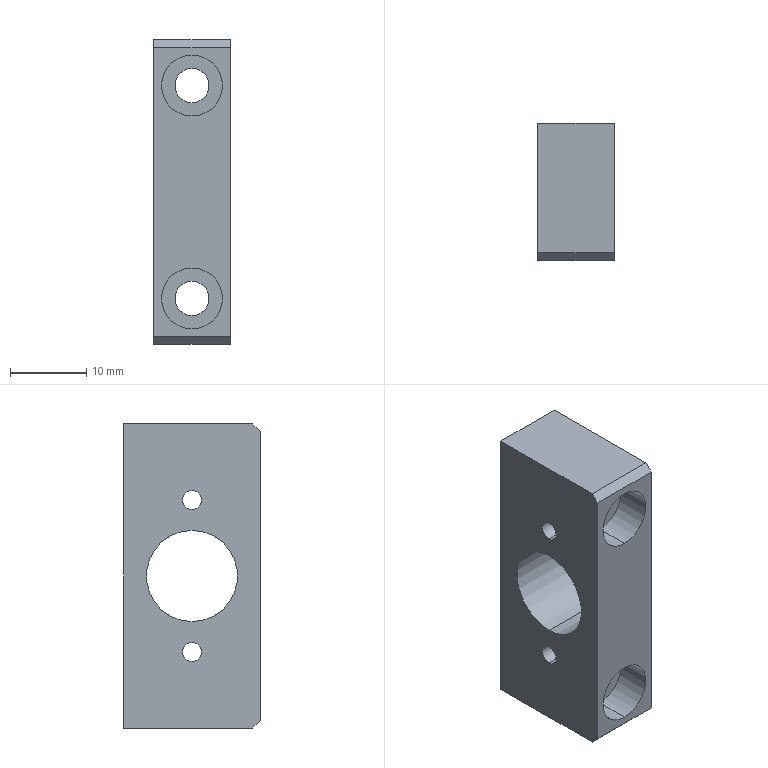Part | STEP file | 0-09-16 Linear bearing mount seat | 1 solid | 24 faces | box 10 x 18 x 40 mm | volume 5072 mm3 | cylinder 14 | plane 10 | commonest cylinder face diameters 2.5 x4 4.5 x4 8 x4 12 x2